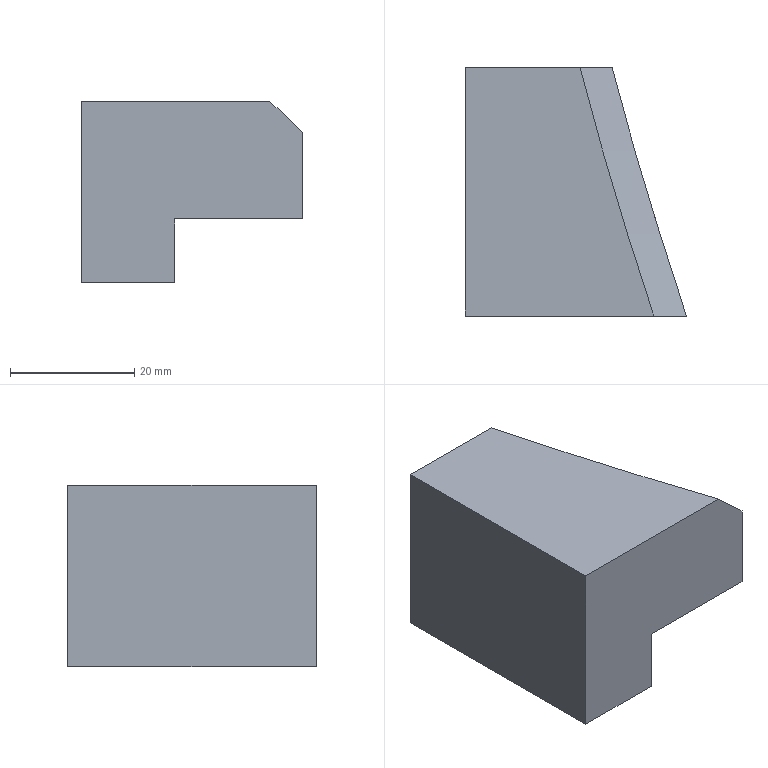Part | STEP file | Positioning_id378_x_t | 1 solid | 9 faces | box 35.628 x 40 x 29.25 mm | volume 27932 mm3 | plane 7 | spline 2
STEP:
#1=CARTESIAN_POINT('',(0.,0.,0.));
#2=DIRECTION('',(0.,0.,1.));
#3=DIRECTION('',(1.,0.,0.));
#4=AXIS2_PLACEMENT_3D('',#1,#2,#3);
#5=CARTESIAN_POINT('',(-770.37,-465.,151.245));
#6=VERTEX_POINT('',#5);
#7=CARTESIAN_POINT('',(-765.202,-465.,146.245));
#8=VERTEX_POINT('',#7);
#9=CARTESIAN_POINT('',(-770.37,-465.,151.245));
#10=CARTESIAN_POINT('',(-769.508,-465.,150.412));
#11=CARTESIAN_POINT('',(-768.647,-465.,149.578));
#12=CARTESIAN_POINT('',(-767.786,-465.,148.745));
#13=CARTESIAN_POINT('',(-766.924,-465.,147.911));
#14=CARTESIAN_POINT('',(-766.063,-465.,147.078));
#15=CARTESIAN_POINT('',(-765.202,-465.,146.245));
#16=B_SPLINE_CURVE_WITH_KNOTS('',3,(#9,#10,#11,#12,#13,#14,#15),.UNSPECIFIED.,.F.,.F.,(4,3,4),(0.,0.5,1.),.UNSPECIFIED.);
#17=CARTESIAN_POINT('',(-765.482,-463.728,146.195));
#18=CARTESIAN_POINT('',(-763.676,-470.672,146.195));
#19=CARTESIAN_POINT('',(-759.81,-484.505,146.195));
#20=CARTESIAN_POINT('',(-755.452,-498.19,146.195));
#21=CARTESIAN_POINT('',(-753.154,-504.984,146.195));
#22=CARTESIAN_POINT('',(-765.498,-463.732,146.212));
#23=CARTESIAN_POINT('',(-763.692,-470.676,146.212));
#24=CARTESIAN_POINT('',(-759.826,-484.51,146.212));
#25=CARTESIAN_POINT('',(-755.468,-498.195,146.212));
#26=CARTESIAN_POINT('',(-753.169,-504.989,146.212));
#27=CARTESIAN_POINT('',(-765.514,-463.737,146.228));
#28=CARTESIAN_POINT('',(-763.708,-470.681,146.228));
#29=CARTESIAN_POINT('',(-759.842,-484.515,146.228));
#30=CARTESIAN_POINT('',(-755.484,-498.2,146.228));
#31=CARTESIAN_POINT('',(-753.185,-504.995,146.228));
#32=CARTESIAN_POINT('',(-765.531,-463.741,146.245));
#33=CARTESIAN_POINT('',(-763.724,-470.685,146.245));
#34=CARTESIAN_POINT('',(-759.858,-484.519,146.245));
#35=CARTESIAN_POINT('',(-755.5,-498.205,146.245));
#36=CARTESIAN_POINT('',(-753.201,-505.,146.245));
#37=CARTESIAN_POINT('',(-767.144,-464.161,147.912));
#38=CARTESIAN_POINT('',(-765.332,-471.124,147.912));
#39=CARTESIAN_POINT('',(-761.455,-484.997,147.912));
#40=CARTESIAN_POINT('',(-757.085,-498.72,147.912));
#41=CARTESIAN_POINT('',(-754.78,-505.534,147.912));
#42=CARTESIAN_POINT('',(-768.757,-464.58,149.578));
#43=CARTESIAN_POINT('',(-766.94,-471.563,149.578));
#44=CARTESIAN_POINT('',(-763.052,-485.474,149.578));
#45=CARTESIAN_POINT('',(-758.67,-499.236,149.578));
#46=CARTESIAN_POINT('',(-756.358,-506.068,149.578));
#47=CARTESIAN_POINT('',(-770.37,-465.,151.245));
#48=CARTESIAN_POINT('',(-768.548,-472.002,151.245));
#49=CARTESIAN_POINT('',(-764.65,-485.951,151.245));
#50=CARTESIAN_POINT('',(-760.255,-499.751,151.245));
#51=CARTESIAN_POINT('',(-757.937,-506.602,151.245));
#52=B_SPLINE_SURFACE_WITH_KNOTS('',3,3,((#17,#18,#19,#20,#21),(#22,#23,#24,#25,#26),(#27,#28,#29,#30,#31),(#32,#33,#34,#35,#36),(#37,#38,#39,#40,#41),(#42,#43,#44,#45,#46),(#47,#48,#49,#50,#51)),.UNSPECIFIED.,.F.,.F.,.F.,(4,3,4),(4,1,4),(0.,0.009901,1.),(0.,0.5,1.),.UNSPECIFIED.);
#53=CARTESIAN_POINT('',(1.,0.));
#54=CARTESIAN_POINT('',(0.009901,0.03023));
#55=B_SPLINE_CURVE_WITH_KNOTS('',1,(#53,#54),.UNSPECIFIED.,.F.,.F.,(2,2),(0.,1.),.PIECEWISE_BEZIER_KNOTS.);
#56=(GEOMETRIC_REPRESENTATION_CONTEXT(2)PARAMETRIC_REPRESENTATION_CONTEXT()REPRESENTATION_CONTEXT('',''));
#57=DEFINITIONAL_REPRESENTATION('',(#55),#56);
#58=PCURVE('',#52,#57);
#59=CARTESIAN_POINT('',(-863.829,-465.,84.282));
#60=DIRECTION('',(0.,1.,0.));
#61=DIRECTION('',(0.,0.,-1.));
#62=AXIS2_PLACEMENT_3D('',#59,#60,#61);
#63=PLANE('',#62);
#64=CARTESIAN_POINT('',(-66.963,-93.459));
#65=CARTESIAN_POINT('',(-66.13,-94.32));
#66=CARTESIAN_POINT('',(-65.296,-95.182));
#67=CARTESIAN_POINT('',(-64.463,-96.043));
#68=CARTESIAN_POINT('',(-63.63,-96.904));
#69=CARTESIAN_POINT('',(-62.796,-97.766));
#70=CARTESIAN_POINT('',(-61.963,-98.627));
#71=B_SPLINE_CURVE_WITH_KNOTS('',3,(#64,#65,#66,#67,#68,#69,#70),.UNSPECIFIED.,.F.,.F.,(4,3,4),(0.,0.5,1.),.UNSPECIFIED.);
#72=(GEOMETRIC_REPRESENTATION_CONTEXT(2)PARAMETRIC_REPRESENTATION_CONTEXT()REPRESENTATION_CONTEXT('',''));
#73=DEFINITIONAL_REPRESENTATION('',(#71),#72);
#74=PCURVE('',#63,#73);
#75=SURFACE_CURVE('',#16,(#58,#74),.PCURVE_S1.);
#76=EDGE_CURVE('',#6,#8,#75,.T.);
#77=ORIENTED_EDGE('',*,*,#76,.F.);
#78=CARTESIAN_POINT('',(-758.477,-505.,151.245));
#79=VERTEX_POINT('',#78);
#80=CARTESIAN_POINT('',(-758.477,-505.,151.245));
#81=CARTESIAN_POINT('',(-760.597,-498.675,151.245));
#82=CARTESIAN_POINT('',(-764.802,-485.408,151.245));
#83=CARTESIAN_POINT('',(-768.548,-472.002,151.245));
#84=CARTESIAN_POINT('',(-770.37,-465.,151.245));
#85=B_SPLINE_CURVE_WITH_KNOTS('',3,(#80,#81,#82,#83,#84),.UNSPECIFIED.,.F.,.F.,(4,1,4),(0.,0.4797,1.),.UNSPECIFIED.);
#86=CARTESIAN_POINT('',(1.,0.961));
#87=CARTESIAN_POINT('',(1.,0.));
#88=B_SPLINE_CURVE_WITH_KNOTS('',1,(#86,#87),.UNSPECIFIED.,.F.,.F.,(2,2),(0.,1.),.PIECEWISE_BEZIER_KNOTS.);
#89=(GEOMETRIC_REPRESENTATION_CONTEXT(2)PARAMETRIC_REPRESENTATION_CONTEXT()REPRESENTATION_CONTEXT('',''));
#90=DEFINITIONAL_REPRESENTATION('',(#88),#89);
#91=PCURVE('',#52,#90);
#92=CARTESIAN_POINT('',(-788.829,-465.,151.245));
#93=DIRECTION('',(0.,0.,-1.));
#94=DIRECTION('',(1.,0.,0.));
#95=AXIS2_PLACEMENT_3D('',#92,#93,#94);
#96=PLANE('',#95);
#97=CARTESIAN_POINT('',(30.352,40.));
#98=CARTESIAN_POINT('',(28.232,33.675));
#99=CARTESIAN_POINT('',(24.027,20.408));
#100=CARTESIAN_POINT('',(20.281,7.002));
#101=CARTESIAN_POINT('',(18.459,-0.000000011));
#102=B_SPLINE_CURVE_WITH_KNOTS('',3,(#97,#98,#99,#100,#101),.UNSPECIFIED.,.F.,.F.,(4,1,4),(0.,0.4797,1.),.UNSPECIFIED.);
#103=(GEOMETRIC_REPRESENTATION_CONTEXT(2)PARAMETRIC_REPRESENTATION_CONTEXT()REPRESENTATION_CONTEXT('',''));
#104=DEFINITIONAL_REPRESENTATION('',(#102),#103);
#105=PCURVE('',#96,#104);
#106=SURFACE_CURVE('',#85,(#91,#105),.PCURVE_S1.);
#107=EDGE_CURVE('',#79,#6,#106,.T.);
#108=ORIENTED_EDGE('',*,*,#107,.F.);
#109=CARTESIAN_POINT('',(-753.201,-505.,146.245));
#110=VERTEX_POINT('',#109);
#111=CARTESIAN_POINT('',(-753.201,-505.,146.245));
#112=CARTESIAN_POINT('',(-754.08,-505.,147.078));
#113=CARTESIAN_POINT('',(-754.96,-505.,147.911));
#114=CARTESIAN_POINT('',(-755.839,-505.,148.745));
#115=CARTESIAN_POINT('',(-756.718,-505.,149.578));
#116=CARTESIAN_POINT('',(-757.598,-505.,150.411));
#117=CARTESIAN_POINT('',(-758.477,-505.,151.245));
#118=B_SPLINE_CURVE_WITH_KNOTS('',3,(#111,#112,#113,#114,#115,#116,#117),.UNSPECIFIED.,.F.,.F.,(4,3,4),(0.,0.5,1.),.UNSPECIFIED.);
#119=CARTESIAN_POINT('',(0.009906,1.));
#120=CARTESIAN_POINT('',(1.,0.961));
#121=B_SPLINE_CURVE_WITH_KNOTS('',1,(#119,#120),.UNSPECIFIED.,.F.,.F.,(2,2),(0.,1.),.PIECEWISE_BEZIER_KNOTS.);
#122=(GEOMETRIC_REPRESENTATION_CONTEXT(2)PARAMETRIC_REPRESENTATION_CONTEXT()REPRESENTATION_CONTEXT('',''));
#123=DEFINITIONAL_REPRESENTATION('',(#121),#122);
#124=PCURVE('',#52,#123);
#125=CARTESIAN_POINT('',(-863.829,-505.,84.282));
#126=DIRECTION('',(0.,-1.,0.));
#127=DIRECTION('',(0.,0.,1.));
#128=AXIS2_PLACEMENT_3D('',#125,#126,#127);
#129=PLANE('',#128);
#130=CARTESIAN_POINT('',(61.963,-110.628));
#131=CARTESIAN_POINT('',(62.796,-109.748));
#132=CARTESIAN_POINT('',(63.629,-108.869));
#133=CARTESIAN_POINT('',(64.463,-107.99));
#134=CARTESIAN_POINT('',(65.296,-107.11));
#135=CARTESIAN_POINT('',(66.13,-106.231));
#136=CARTESIAN_POINT('',(66.963,-105.352));
#137=B_SPLINE_CURVE_WITH_KNOTS('',3,(#130,#131,#132,#133,#134,#135,#136),.UNSPECIFIED.,.F.,.F.,(4,3,4),(0.,0.5,1.),.UNSPECIFIED.);
#138=(GEOMETRIC_REPRESENTATION_CONTEXT(2)PARAMETRIC_REPRESENTATION_CONTEXT()REPRESENTATION_CONTEXT('',''));
#139=DEFINITIONAL_REPRESENTATION('',(#137),#138);
#140=PCURVE('',#129,#139);
#141=SURFACE_CURVE('',#118,(#124,#140),.PCURVE_S1.);
#142=EDGE_CURVE('',#110,#79,#141,.T.);
#143=ORIENTED_EDGE('',*,*,#142,.F.);
#144=CARTESIAN_POINT('',(-765.202,-465.,146.245));
#145=CARTESIAN_POINT('',(-764.004,-469.56,146.245));
#146=CARTESIAN_POINT('',(-762.753,-474.107,146.245));
#147=CARTESIAN_POINT('',(-761.449,-478.638,146.245));
#148=CARTESIAN_POINT('',(-760.176,-483.061,146.245));
#149=CARTESIAN_POINT('',(-758.852,-487.47,146.245));
#150=CARTESIAN_POINT('',(-757.478,-491.863,146.245));
#151=CARTESIAN_POINT('',(-756.102,-496.258,146.245));
#152=CARTESIAN_POINT('',(-754.677,-500.638,146.245));
#153=CARTESIAN_POINT('',(-753.201,-505.,146.245));
#154=B_SPLINE_CURVE_WITH_KNOTS('',3,(#144,#145,#146,#147,#148,#149,#150,#151,#152,#153),.UNSPECIFIED.,.F.,.F.,(4,3,3,4),(0.,0.3386,0.6692,1.),.UNSPECIFIED.);
#155=CARTESIAN_POINT('',(0.009894,0.03023));
#156=CARTESIAN_POINT('',(0.009903,1.));
#157=B_SPLINE_CURVE_WITH_KNOTS('',1,(#155,#156),.UNSPECIFIED.,.F.,.F.,(2,2),(0.,1.),.PIECEWISE_BEZIER_KNOTS.);
#158=(GEOMETRIC_REPRESENTATION_CONTEXT(2)PARAMETRIC_REPRESENTATION_CONTEXT()REPRESENTATION_CONTEXT('',''));
#159=DEFINITIONAL_REPRESENTATION('',(#157),#158);
#160=PCURVE('',#52,#159);
#161=CARTESIAN_POINT('',(-753.201,-505.,146.385));
#162=CARTESIAN_POINT('',(-753.201,-505.,146.245));
#163=CARTESIAN_POINT('',(-753.201,-505.,132.282));
#164=CARTESIAN_POINT('',(-757.663,-491.811,146.385));
#165=CARTESIAN_POINT('',(-757.663,-491.811,146.245));
#166=CARTESIAN_POINT('',(-757.663,-491.811,132.282));
#167=CARTESIAN_POINT('',(-761.665,-478.472,146.385));
#168=CARTESIAN_POINT('',(-761.665,-478.472,146.245));
#169=CARTESIAN_POINT('',(-761.665,-478.472,132.282));
#170=CARTESIAN_POINT('',(-765.202,-465.,146.385));
#171=CARTESIAN_POINT('',(-765.202,-465.,146.245));
#172=CARTESIAN_POINT('',(-765.202,-465.,132.282));
#173=CARTESIAN_POINT('',(-765.237,-464.865,146.385));
#174=CARTESIAN_POINT('',(-765.237,-464.865,146.245));
#175=CARTESIAN_POINT('',(-765.237,-464.865,132.282));
#176=CARTESIAN_POINT('',(-765.272,-464.731,146.385));
#177=CARTESIAN_POINT('',(-765.272,-464.731,146.245));
#178=CARTESIAN_POINT('',(-765.272,-464.731,132.282));
#179=CARTESIAN_POINT('',(-765.308,-464.596,146.385));
#180=CARTESIAN_POINT('',(-765.308,-464.596,146.245));
#181=CARTESIAN_POINT('',(-765.308,-464.596,132.282));
#182=(BOUNDED_SURFACE()B_SPLINE_SURFACE(3,1,((#161,#162,#163),(#164,#165,#166),(#167,#168,#169),(#170,#171,#172),(#173,#174,#175),(#176,#177,#178),(#179,#180,#181)),.UNSPECIFIED.,.F.,.F.,.F.)B_SPLINE_SURFACE_WITH_KNOTS((4,3,4),(2,1,2),(0.,0.9901,1.),(0.,0.009901,1.),.UNSPECIFIED.)GEOMETRIC_REPRESENTATION_ITEM()RATIONAL_B_SPLINE_SURFACE(((0.9919,0.9919,0.9919),(0.9912,0.9912,0.9912),(0.9909,0.9909,0.9909),(0.9909,0.9909,0.9909),(0.9909,0.9909,0.9909),(0.9909,0.9909,0.9909),(0.9909,0.9909,0.9909)))REPRESENTATION_ITEM('')SURFACE());
#183=CARTESIAN_POINT('',(0.9901,0.009906));
#184=CARTESIAN_POINT('',(0.,0.009903));
#185=B_SPLINE_CURVE_WITH_KNOTS('',1,(#183,#184),.UNSPECIFIED.,.F.,.F.,(2,2),(0.,1.),.PIECEWISE_BEZIER_KNOTS.);
#186=(GEOMETRIC_REPRESENTATION_CONTEXT(2)PARAMETRIC_REPRESENTATION_CONTEXT()REPRESENTATION_CONTEXT('',''));
#187=DEFINITIONAL_REPRESENTATION('',(#185),#186);
#188=PCURVE('',#182,#187);
#189=SURFACE_CURVE('',#154,(#160,#188),.PCURVE_S1.);
#190=EDGE_CURVE('',#8,#110,#189,.T.);
#191=ORIENTED_EDGE('',*,*,#190,.F.);
#192=EDGE_LOOP('',(#77,#108,#143,#191));
#193=FACE_BOUND('',#192,.T.);
#194=ADVANCED_FACE('',(#193),#52,.T.);
#195=CARTESIAN_POINT('',(-788.829,-465.,151.245));
#196=VERTEX_POINT('',#195);
#197=CARTESIAN_POINT('',(-788.829,-505.,151.245));
#198=VERTEX_POINT('',#197);
#199=CARTESIAN_POINT('',(-788.829,-465.,151.245));
#200=DIRECTION('',(0.,-1.,0.));
#201=VECTOR('',#200,1.);
#202=LINE('',#199,#201);
#203=CARTESIAN_POINT('',(0.,0.));
#204=DIRECTION('',(0.,1.));
#205=VECTOR('',#204,1.);
#206=LINE('',#203,#205);
#207=(GEOMETRIC_REPRESENTATION_CONTEXT(2)PARAMETRIC_REPRESENTATION_CONTEXT()REPRESENTATION_CONTEXT('',''));
#208=DEFINITIONAL_REPRESENTATION('',(#206),#207);
#209=PCURVE('',#96,#208);
#210=CARTESIAN_POINT('',(-788.829,-493.037,84.282));
#211=DIRECTION('',(-1.,0.,0.));
#212=DIRECTION('',(0.,0.,-1.));
#213=AXIS2_PLACEMENT_3D('',#210,#211,#212);
#214=PLANE('',#213);
#215=CARTESIAN_POINT('',(-66.963,-28.037));
#216=DIRECTION('',(0.,1.));
#217=VECTOR('',#216,1.);
#218=LINE('',#215,#217);
#219=(GEOMETRIC_REPRESENTATION_CONTEXT(2)PARAMETRIC_REPRESENTATION_CONTEXT()REPRESENTATION_CONTEXT('',''));
#220=DEFINITIONAL_REPRESENTATION('',(#218),#219);
#221=PCURVE('',#214,#220);
#222=SURFACE_CURVE('',#202,(#209,#221),.PCURVE_S1.);
#223=EDGE_CURVE('',#196,#198,#222,.T.);
#224=ORIENTED_EDGE('',*,*,#223,.F.);
#225=CARTESIAN_POINT('',(-770.37,-465.,151.245));
#226=DIRECTION('',(-1.,0.,0.));
#227=VECTOR('',#226,1.);
#228=LINE('',#225,#227);
#229=CARTESIAN_POINT('',(18.459,0.));
#230=DIRECTION('',(-1.,0.));
#231=VECTOR('',#230,1.);
#232=LINE('',#229,#231);
#233=(GEOMETRIC_REPRESENTATION_CONTEXT(2)PARAMETRIC_REPRESENTATION_CONTEXT()REPRESENTATION_CONTEXT('',''));
#234=DEFINITIONAL_REPRESENTATION('',(#232),#233);
#235=PCURVE('',#96,#234);
#236=CARTESIAN_POINT('',(-66.963,-93.459));
#237=DIRECTION('',(0.,1.));
#238=VECTOR('',#237,1.);
#239=LINE('',#236,#238);
#240=(GEOMETRIC_REPRESENTATION_CONTEXT(2)PARAMETRIC_REPRESENTATION_CONTEXT()REPRESENTATION_CONTEXT('',''));
#241=DEFINITIONAL_REPRESENTATION('',(#239),#240);
#242=PCURVE('',#63,#241);
#243=SURFACE_CURVE('',#228,(#235,#242),.PCURVE_S1.);
#244=EDGE_CURVE('',#6,#196,#243,.T.);
#245=ORIENTED_EDGE('',*,*,#244,.F.);
#246=ORIENTED_EDGE('',*,*,#107,.F.);
#247=CARTESIAN_POINT('',(-788.829,-505.,151.245));
#248=DIRECTION('',(1.,0.,0.));
#249=VECTOR('',#248,1.);
#250=LINE('',#247,#249);
#251=CARTESIAN_POINT('',(0.,40.));
#252=DIRECTION('',(1.,0.));
#253=VECTOR('',#252,1.);
#254=LINE('',#251,#253);
#255=(GEOMETRIC_REPRESENTATION_CONTEXT(2)PARAMETRIC_REPRESENTATION_CONTEXT()REPRESENTATION_CONTEXT('',''));
#256=DEFINITIONAL_REPRESENTATION('',(#254),#255);
#257=PCURVE('',#96,#256);
#258=CARTESIAN_POINT('',(66.963,-75.));
#259=DIRECTION('',(0.,-1.));
#260=VECTOR('',#259,1.);
#261=LINE('',#258,#260);
#262=(GEOMETRIC_REPRESENTATION_CONTEXT(2)PARAMETRIC_REPRESENTATION_CONTEXT()REPRESENTATION_CONTEXT('',''));
#263=DEFINITIONAL_REPRESENTATION('',(#261),#262);
#264=PCURVE('',#129,#263);
#265=SURFACE_CURVE('',#250,(#257,#264),.PCURVE_S1.);
#266=EDGE_CURVE('',#198,#79,#265,.T.);
#267=ORIENTED_EDGE('',*,*,#266,.F.);
#268=EDGE_LOOP('',(#224,#245,#246,#267));
#269=FACE_BOUND('',#268,.F.);
#270=ADVANCED_FACE('',(#269),#96,.F.);
#271=CARTESIAN_POINT('',(-753.201,-505.,132.282));
#272=VERTEX_POINT('',#271);
#273=CARTESIAN_POINT('',(-765.202,-465.,132.282));
#274=VERTEX_POINT('',#273);
#275=CARTESIAN_POINT('',(-753.201,-505.,132.282));
#276=CARTESIAN_POINT('',(-757.663,-491.811,132.282));
#277=CARTESIAN_POINT('',(-761.665,-478.472,132.282));
#278=CARTESIAN_POINT('',(-765.202,-465.,132.282));
#279=(BOUNDED_CURVE()B_SPLINE_CURVE(3,(#275,#276,#277,#278),.UNSPECIFIED.,.F.,.F.)B_SPLINE_CURVE_WITH_KNOTS((4,4),(0.,1.),.PIECEWISE_BEZIER_KNOTS.)CURVE()GEOMETRIC_REPRESENTATION_ITEM()RATIONAL_B_SPLINE_CURVE((0.9919,0.9912,0.9909,0.9909))REPRESENTATION_ITEM(''));
#280=CARTESIAN_POINT('',(0.,1.));
#281=CARTESIAN_POINT('',(0.9901,1.));
#282=B_SPLINE_CURVE_WITH_KNOTS('',1,(#280,#281),.UNSPECIFIED.,.F.,.F.,(2,2),(0.,1.),.PIECEWISE_BEZIER_KNOTS.);
#283=(GEOMETRIC_REPRESENTATION_CONTEXT(2)PARAMETRIC_REPRESENTATION_CONTEXT()REPRESENTATION_CONTEXT('',''));
#284=DEFINITIONAL_REPRESENTATION('',(#282),#283);
#285=PCURVE('',#182,#284);
#286=CARTESIAN_POINT('',(-853.829,-493.037,132.282));
#287=DIRECTION('',(0.,0.,-1.));
#288=DIRECTION('',(1.,0.,0.));
#289=AXIS2_PLACEMENT_3D('',#286,#287,#288);
#290=PLANE('',#289);
#291=CARTESIAN_POINT('',(100.628,11.963));
#292=CARTESIAN_POINT('',(96.166,-1.226));
#293=CARTESIAN_POINT('',(92.164,-14.565));
#294=CARTESIAN_POINT('',(88.627,-28.037));
#295=(BOUNDED_CURVE()B_SPLINE_CURVE(3,(#291,#292,#293,#294),.UNSPECIFIED.,.F.,.F.)B_SPLINE_CURVE_WITH_KNOTS((4,4),(0.,1.),.PIECEWISE_BEZIER_KNOTS.)CURVE()GEOMETRIC_REPRESENTATION_ITEM()RATIONAL_B_SPLINE_CURVE((0.9919,0.9912,0.9909,0.9909))REPRESENTATION_ITEM(''));
#296=(GEOMETRIC_REPRESENTATION_CONTEXT(2)PARAMETRIC_REPRESENTATION_CONTEXT()REPRESENTATION_CONTEXT('',''));
#297=DEFINITIONAL_REPRESENTATION('',(#295),#296);
#298=PCURVE('',#290,#297);
#299=SURFACE_CURVE('',#279,(#285,#298),.PCURVE_S1.);
#300=EDGE_CURVE('',#272,#274,#299,.T.);
#301=ORIENTED_EDGE('',*,*,#300,.F.);
#302=CARTESIAN_POINT('',(-753.201,-505.,146.245));
#303=DIRECTION('',(0.,0.,-1.));
#304=VECTOR('',#303,1.);
#305=LINE('',#302,#304);
#306=CARTESIAN_POINT('',(0.,0.009901));
#307=CARTESIAN_POINT('',(0.,1.));
#308=B_SPLINE_CURVE_WITH_KNOTS('',1,(#306,#307),.UNSPECIFIED.,.F.,.F.,(2,2),(0.,13.963),.PIECEWISE_BEZIER_KNOTS.);
#309=(GEOMETRIC_REPRESENTATION_CONTEXT(2)PARAMETRIC_REPRESENTATION_CONTEXT()REPRESENTATION_CONTEXT('',''));
#310=DEFINITIONAL_REPRESENTATION('',(#308),#309);
#311=PCURVE('',#182,#310);
#312=CARTESIAN_POINT('',(61.963,-110.628));
#313=DIRECTION('',(-1.,0.));
#314=VECTOR('',#313,1.);
#315=LINE('',#312,#314);
#316=(GEOMETRIC_REPRESENTATION_CONTEXT(2)PARAMETRIC_REPRESENTATION_CONTEXT()REPRESENTATION_CONTEXT('',''));
#317=DEFINITIONAL_REPRESENTATION('',(#315),#316);
#318=PCURVE('',#129,#317);
#319=SURFACE_CURVE('',#305,(#311,#318),.PCURVE_S1.);
#320=EDGE_CURVE('',#110,#272,#319,.T.);
#321=ORIENTED_EDGE('',*,*,#320,.F.);
#322=ORIENTED_EDGE('',*,*,#190,.F.);
#323=CARTESIAN_POINT('',(-765.202,-465.,132.282));
#324=DIRECTION('',(0.,0.,1.));
#325=VECTOR('',#324,1.);
#326=LINE('',#323,#325);
#327=CARTESIAN_POINT('',(0.9901,1.));
#328=CARTESIAN_POINT('',(0.9901,0.009904));
#329=B_SPLINE_CURVE_WITH_KNOTS('',1,(#327,#328),.UNSPECIFIED.,.F.,.F.,(2,2),(0.,13.963),.PIECEWISE_BEZIER_KNOTS.);
#330=(GEOMETRIC_REPRESENTATION_CONTEXT(2)PARAMETRIC_REPRESENTATION_CONTEXT()REPRESENTATION_CONTEXT('',''));
#331=DEFINITIONAL_REPRESENTATION('',(#329),#330);
#332=PCURVE('',#182,#331);
#333=CARTESIAN_POINT('',(-48.,-98.627));
#334=DIRECTION('',(-1.,0.));
#335=VECTOR('',#334,1.);
#336=LINE('',#333,#335);
#337=(GEOMETRIC_REPRESENTATION_CONTEXT(2)PARAMETRIC_REPRESENTATION_CONTEXT()REPRESENTATION_CONTEXT('',''));
#338=DEFINITIONAL_REPRESENTATION('',(#336),#337);
#339=PCURVE('',#63,#338);
#340=SURFACE_CURVE('',#326,(#332,#339),.PCURVE_S1.);
#341=EDGE_CURVE('',#274,#8,#340,.T.);
#342=ORIENTED_EDGE('',*,*,#341,.F.);
#343=EDGE_LOOP('',(#301,#321,#322,#342));
#344=FACE_BOUND('',#343,.F.);
#345=ADVANCED_FACE('',(#344),#182,.F.);
#346=ORIENTED_EDGE('',*,*,#300,.F.);
#347=CARTESIAN_POINT('',(-773.829,-505.,132.282));
#348=VERTEX_POINT('',#347);
#349=CARTESIAN_POINT('',(-773.829,-505.,132.282));
#350=DIRECTION('',(1.,0.,0.));
#351=VECTOR('',#350,1.);
#352=LINE('',#349,#351);
#353=CARTESIAN_POINT('',(80.,11.963));
#354=DIRECTION('',(1.,0.));
#355=VECTOR('',#354,1.);
#356=LINE('',#353,#355);
#357=(GEOMETRIC_REPRESENTATION_CONTEXT(2)PARAMETRIC_REPRESENTATION_CONTEXT()REPRESENTATION_CONTEXT('',''));
#358=DEFINITIONAL_REPRESENTATION('',(#356),#357);
#359=PCURVE('',#290,#358);
#360=CARTESIAN_POINT('',(48.,-90.));
#361=DIRECTION('',(0.,-1.));
#362=VECTOR('',#361,1.);
#363=LINE('',#360,#362);
#364=(GEOMETRIC_REPRESENTATION_CONTEXT(2)PARAMETRIC_REPRESENTATION_CONTEXT()REPRESENTATION_CONTEXT('',''));
#365=DEFINITIONAL_REPRESENTATION('',(#363),#364);
#366=PCURVE('',#129,#365);
#367=SURFACE_CURVE('',#352,(#359,#366),.PCURVE_S1.);
#368=EDGE_CURVE('',#348,#272,#367,.T.);
#369=ORIENTED_EDGE('',*,*,#368,.F.);
#370=CARTESIAN_POINT('',(-773.829,-465.,132.282));
#371=VERTEX_POINT('',#370);
#372=CARTESIAN_POINT('',(-773.829,-505.,132.282));
#373=DIRECTION('',(0.,1.,0.));
#374=VECTOR('',#373,1.);
#375=LINE('',#372,#374);
#376=CARTESIAN_POINT('',(80.,11.963));
#377=DIRECTION('',(0.,-1.));
#378=VECTOR('',#377,1.);
#379=LINE('',#376,#378);
#380=(GEOMETRIC_REPRESENTATION_CONTEXT(2)PARAMETRIC_REPRESENTATION_CONTEXT()REPRESENTATION_CONTEXT('',''));
#381=DEFINITIONAL_REPRESENTATION('',(#379),#380);
#382=PCURVE('',#290,#381);
#383=CARTESIAN_POINT('',(-773.829,-463.037,135.282));
#384=DIRECTION('',(1.,0.,0.));
#385=DIRECTION('',(0.,0.,1.));
#386=AXIS2_PLACEMENT_3D('',#383,#384,#385);
#387=PLANE('',#386);
#388=CARTESIAN_POINT('',(-3.,41.963));
#389=DIRECTION('',(0.,-1.));
#390=VECTOR('',#389,1.);
#391=LINE('',#388,#390);
#392=(GEOMETRIC_REPRESENTATION_CONTEXT(2)PARAMETRIC_REPRESENTATION_CONTEXT()REPRESENTATION_CONTEXT('',''));
#393=DEFINITIONAL_REPRESENTATION('',(#391),#392);
#394=PCURVE('',#387,#393);
#395=SURFACE_CURVE('',#375,(#382,#394),.PCURVE_S1.);
#396=EDGE_CURVE('',#348,#371,#395,.T.);
#397=ORIENTED_EDGE('',*,*,#396,.T.);
#398=CARTESIAN_POINT('',(-765.202,-465.,132.282));
#399=DIRECTION('',(-1.,0.,0.));
#400=VECTOR('',#399,1.);
#401=LINE('',#398,#400);
#402=CARTESIAN_POINT('',(88.627,-28.037));
#403=DIRECTION('',(-1.,0.));
#404=VECTOR('',#403,1.);
#405=LINE('',#402,#404);
#406=(GEOMETRIC_REPRESENTATION_CONTEXT(2)PARAMETRIC_REPRESENTATION_CONTEXT()REPRESENTATION_CONTEXT('',''));
#407=DEFINITIONAL_REPRESENTATION('',(#405),#406);
#408=PCURVE('',#290,#407);
#409=CARTESIAN_POINT('',(-48.,-98.627));
#410=DIRECTION('',(0.,1.));
#411=VECTOR('',#410,1.);
#412=LINE('',#409,#411);
#413=(GEOMETRIC_REPRESENTATION_CONTEXT(2)PARAMETRIC_REPRESENTATION_CONTEXT()REPRESENTATION_CONTEXT('',''));
#414=DEFINITIONAL_REPRESENTATION('',(#412),#413);
#415=PCURVE('',#63,#414);
#416=SURFACE_CURVE('',#401,(#408,#415),.PCURVE_S1.);
#417=EDGE_CURVE('',#274,#371,#416,.T.);
#418=ORIENTED_EDGE('',*,*,#417,.F.);
#419=EDGE_LOOP('',(#346,#369,#397,#418));
#420=FACE_BOUND('',#419,.T.);
#421=ADVANCED_FACE('',(#420),#290,.T.);
#422=CARTESIAN_POINT('',(-788.829,-465.,121.995));
#423=VERTEX_POINT('',#422);
#424=CARTESIAN_POINT('',(-788.829,-465.,121.995));
#425=DIRECTION('',(0.,0.,1.));
#426=VECTOR('',#425,1.);
#427=LINE('',#424,#426);
#428=CARTESIAN_POINT('',(-37.713,-28.037));
#429=DIRECTION('',(-1.,0.));
#430=VECTOR('',#429,1.);
#431=LINE('',#428,#430);
#432=(GEOMETRIC_REPRESENTATION_CONTEXT(2)PARAMETRIC_REPRESENTATION_CONTEXT()REPRESENTATION_CONTEXT('',''));
#433=DEFINITIONAL_REPRESENTATION('',(#431),#432);
#434=PCURVE('',#214,#433);
#435=CARTESIAN_POINT('',(-37.713,-75.));
#436=DIRECTION('',(-1.,0.));
#437=VECTOR('',#436,1.);
#438=LINE('',#435,#437);
#439=(GEOMETRIC_REPRESENTATION_CONTEXT(2)PARAMETRIC_REPRESENTATION_CONTEXT()REPRESENTATION_CONTEXT('',''));
#440=DEFINITIONAL_REPRESENTATION('',(#438),#439);
#441=PCURVE('',#63,#440);
#442=SURFACE_CURVE('',#427,(#434,#441),.PCURVE_S1.);
#443=EDGE_CURVE('',#423,#196,#442,.T.);
#444=ORIENTED_EDGE('',*,*,#443,.F.);
#445=CARTESIAN_POINT('',(-788.829,-505.,121.995));
#446=VERTEX_POINT('',#445);
#447=CARTESIAN_POINT('',(-788.829,-505.,121.995));
#448=DIRECTION('',(0.,1.,0.));
#449=VECTOR('',#448,1.);
#450=LINE('',#447,#449);
#451=CARTESIAN_POINT('',(-37.713,11.963));
#452=DIRECTION('',(0.,-1.));
#453=VECTOR('',#452,1.);
#454=LINE('',#451,#453);
#455=(GEOMETRIC_REPRESENTATION_CONTEXT(2)PARAMETRIC_REPRESENTATION_CONTEXT()REPRESENTATION_CONTEXT('',''));
#456=DEFINITIONAL_REPRESENTATION('',(#454),#455);
#457=PCURVE('',#214,#456);
#458=CARTESIAN_POINT('',(-843.829,-463.037,121.995));
#459=DIRECTION('',(0.,0.,1.));
#460=DIRECTION('',(-1.,0.,0.));
#461=AXIS2_PLACEMENT_3D('',#458,#459,#460);
#462=PLANE('',#461);
#463=CARTESIAN_POINT('',(-55.,41.963));
#464=DIRECTION('',(0.,-1.));
#465=VECTOR('',#464,1.);
#466=LINE('',#463,#465);
#467=(GEOMETRIC_REPRESENTATION_CONTEXT(2)PARAMETRIC_REPRESENTATION_CONTEXT()REPRESENTATION_CONTEXT('',''));
#468=DEFINITIONAL_REPRESENTATION('',(#466),#467);
#469=PCURVE('',#462,#468);
#470=SURFACE_CURVE('',#450,(#457,#469),.PCURVE_S1.);
#471=EDGE_CURVE('',#446,#423,#470,.T.);
#472=ORIENTED_EDGE('',*,*,#471,.F.);
#473=CARTESIAN_POINT('',(-788.829,-505.,151.245));
#474=DIRECTION('',(0.,0.,-1.));
#475=VECTOR('',#474,1.);
#476=LINE('',#473,#475);
#477=CARTESIAN_POINT('',(-66.963,11.963));
#478=DIRECTION('',(1.,0.));
#479=VECTOR('',#478,1.);
#480=LINE('',#477,#479);
#481=(GEOMETRIC_REPRESENTATION_CONTEXT(2)PARAMETRIC_REPRESENTATION_CONTEXT()REPRESENTATION_CONTEXT('',''));
#482=DEFINITIONAL_REPRESENTATION('',(#480),#481);
#483=PCURVE('',#214,#482);
#484=CARTESIAN_POINT('',(66.963,-75.));
#485=DIRECTION('',(-1.,0.));
#486=VECTOR('',#485,1.);
#487=LINE('',#484,#486);
#488=(GEOMETRIC_REPRESENTATION_CONTEXT(2)PARAMETRIC_REPRESENTATION_CONTEXT()REPRESENTATION_CONTEXT('',''));
#489=DEFINITIONAL_REPRESENTATION('',(#487),#488);
#490=PCURVE('',#129,#489);
#491=SURFACE_CURVE('',#476,(#483,#490),.PCURVE_S1.);
#492=EDGE_CURVE('',#198,#446,#491,.T.);
#493=ORIENTED_EDGE('',*,*,#492,.F.);
#494=ORIENTED_EDGE('',*,*,#223,.F.);
#495=EDGE_LOOP('',(#444,#472,#493,#494));
#496=FACE_BOUND('',#495,.T.);
#497=ADVANCED_FACE('',(#496),#214,.T.);
#498=ORIENTED_EDGE('',*,*,#396,.F.);
#499=CARTESIAN_POINT('',(-773.829,-505.,121.995));
#500=VERTEX_POINT('',#499);
#501=CARTESIAN_POINT('',(-773.829,-505.,121.995));
#502=DIRECTION('',(0.,0.,1.));
#503=VECTOR('',#502,1.);
#504=LINE('',#501,#503);
#505=CARTESIAN_POINT('',(-13.287,41.963));
#506=DIRECTION('',(1.,0.));
#507=VECTOR('',#506,1.);
#508=LINE('',#505,#507);
#509=(GEOMETRIC_REPRESENTATION_CONTEXT(2)PARAMETRIC_REPRESENTATION_CONTEXT()REPRESENTATION_CONTEXT('',''));
#510=DEFINITIONAL_REPRESENTATION('',(#508),#509);
#511=PCURVE('',#387,#510);
#512=CARTESIAN_POINT('',(37.713,-90.));
#513=DIRECTION('',(1.,0.));
#514=VECTOR('',#513,1.);
#515=LINE('',#512,#514);
#516=(GEOMETRIC_REPRESENTATION_CONTEXT(2)PARAMETRIC_REPRESENTATION_CONTEXT()REPRESENTATION_CONTEXT('',''));
#517=DEFINITIONAL_REPRESENTATION('',(#515),#516);
#518=PCURVE('',#129,#517);
#519=SURFACE_CURVE('',#504,(#511,#518),.PCURVE_S1.);
#520=EDGE_CURVE('',#500,#348,#519,.T.);
#521=ORIENTED_EDGE('',*,*,#520,.F.);
#522=CARTESIAN_POINT('',(-773.829,-465.,121.995));
#523=VERTEX_POINT('',#522);
#524=CARTESIAN_POINT('',(-773.829,-465.,121.995));
#525=DIRECTION('',(0.,-1.,0.));
#526=VECTOR('',#525,1.);
#527=LINE('',#524,#526);
#528=CARTESIAN_POINT('',(-13.287,1.963));
#529=DIRECTION('',(0.,1.));
#530=VECTOR('',#529,1.);
#531=LINE('',#528,#530);
#532=(GEOMETRIC_REPRESENTATION_CONTEXT(2)PARAMETRIC_REPRESENTATION_CONTEXT()REPRESENTATION_CONTEXT('',''));
#533=DEFINITIONAL_REPRESENTATION('',(#531),#532);
#534=PCURVE('',#387,#533);
#535=CARTESIAN_POINT('',(-70.,1.963));
#536=DIRECTION('',(0.,1.));
#537=VECTOR('',#536,1.);
#538=LINE('',#535,#537);
#539=(GEOMETRIC_REPRESENTATION_CONTEXT(2)PARAMETRIC_REPRESENTATION_CONTEXT()REPRESENTATION_CONTEXT('',''));
#540=DEFINITIONAL_REPRESENTATION('',(#538),#539);
#541=PCURVE('',#462,#540);
#542=SURFACE_CURVE('',#527,(#534,#541),.PCURVE_S1.);
#543=EDGE_CURVE('',#523,#500,#542,.T.);
#544=ORIENTED_EDGE('',*,*,#543,.F.);
#545=CARTESIAN_POINT('',(-773.829,-465.,132.282));
#546=DIRECTION('',(0.,0.,-1.));
#547=VECTOR('',#546,1.);
#548=LINE('',#545,#547);
#549=CARTESIAN_POINT('',(-3.,1.963));
#550=DIRECTION('',(-1.,0.));
#551=VECTOR('',#550,1.);
#552=LINE('',#549,#551);
#553=(GEOMETRIC_REPRESENTATION_CONTEXT(2)PARAMETRIC_REPRESENTATION_CONTEXT()REPRESENTATION_CONTEXT('',''));
#554=DEFINITIONAL_REPRESENTATION('',(#552),#553);
#555=PCURVE('',#387,#554);
#556=CARTESIAN_POINT('',(-48.,-90.));
#557=DIRECTION('',(1.,0.));
#558=VECTOR('',#557,1.);
#559=LINE('',#556,#558);
#560=(GEOMETRIC_REPRESENTATION_CONTEXT(2)PARAMETRIC_REPRESENTATION_CONTEXT()REPRESENTATION_CONTEXT('',''));
#561=DEFINITIONAL_REPRESENTATION('',(#559),#560);
#562=PCURVE('',#63,#561);
#563=SURFACE_CURVE('',#548,(#555,#562),.PCURVE_S1.);
#564=EDGE_CURVE('',#371,#523,#563,.T.);
#565=ORIENTED_EDGE('',*,*,#564,.F.);
#566=EDGE_LOOP('',(#498,#521,#544,#565));
#567=FACE_BOUND('',#566,.T.);
#568=ADVANCED_FACE('',(#567),#387,.T.);
#569=ORIENTED_EDGE('',*,*,#492,.T.);
#570=CARTESIAN_POINT('',(-773.829,-505.,121.995));
#571=DIRECTION('',(-1.,0.,0.));
#572=VECTOR('',#571,1.);
#573=LINE('',#570,#572);
#574=CARTESIAN_POINT('',(37.713,-90.));
#575=DIRECTION('',(0.,1.));
#576=VECTOR('',#575,1.);
#577=LINE('',#574,#576);
#578=(GEOMETRIC_REPRESENTATION_CONTEXT(2)PARAMETRIC_REPRESENTATION_CONTEXT()REPRESENTATION_CONTEXT('',''));
#579=DEFINITIONAL_REPRESENTATION('',(#577),#578);
#580=PCURVE('',#129,#579);
#581=CARTESIAN_POINT('',(-70.,41.963));
#582=DIRECTION('',(1.,0.));
#583=VECTOR('',#582,1.);
#584=LINE('',#581,#583);
#585=(GEOMETRIC_REPRESENTATION_CONTEXT(2)PARAMETRIC_REPRESENTATION_CONTEXT()REPRESENTATION_CONTEXT('',''));
#586=DEFINITIONAL_REPRESENTATION('',(#584),#585);
#587=PCURVE('',#462,#586);
#588=SURFACE_CURVE('',#573,(#580,#587),.PCURVE_S1.);
#589=EDGE_CURVE('',#500,#446,#588,.T.);
#590=ORIENTED_EDGE('',*,*,#589,.F.);
#591=ORIENTED_EDGE('',*,*,#520,.T.);
#592=ORIENTED_EDGE('',*,*,#368,.T.);
#593=ORIENTED_EDGE('',*,*,#320,.F.);
#594=ORIENTED_EDGE('',*,*,#142,.T.);
#595=ORIENTED_EDGE('',*,*,#266,.F.);
#596=EDGE_LOOP('',(#569,#590,#591,#592,#593,#594,#595));
#597=FACE_BOUND('',#596,.T.);
#598=ADVANCED_FACE('',(#597),#129,.T.);
#599=CARTESIAN_POINT('',(-788.829,-465.,121.995));
#600=DIRECTION('',(1.,0.,0.));
#601=VECTOR('',#600,1.);
#602=LINE('',#599,#601);
#603=CARTESIAN_POINT('',(-37.713,-75.));
#604=DIRECTION('',(0.,-1.));
#605=VECTOR('',#604,1.);
#606=LINE('',#603,#605);
#607=(GEOMETRIC_REPRESENTATION_CONTEXT(2)PARAMETRIC_REPRESENTATION_CONTEXT()REPRESENTATION_CONTEXT('',''));
#608=DEFINITIONAL_REPRESENTATION('',(#606),#607);
#609=PCURVE('',#63,#608);
#610=CARTESIAN_POINT('',(-55.,1.963));
#611=DIRECTION('',(-1.,0.));
#612=VECTOR('',#611,1.);
#613=LINE('',#610,#612);
#614=(GEOMETRIC_REPRESENTATION_CONTEXT(2)PARAMETRIC_REPRESENTATION_CONTEXT()REPRESENTATION_CONTEXT('',''));
#615=DEFINITIONAL_REPRESENTATION('',(#613),#614);
#616=PCURVE('',#462,#615);
#617=SURFACE_CURVE('',#602,(#609,#616),.PCURVE_S1.);
#618=EDGE_CURVE('',#423,#523,#617,.T.);
#619=ORIENTED_EDGE('',*,*,#618,.F.);
#620=ORIENTED_EDGE('',*,*,#443,.T.);
#621=ORIENTED_EDGE('',*,*,#244,.F.);
#622=ORIENTED_EDGE('',*,*,#76,.T.);
#623=ORIENTED_EDGE('',*,*,#341,.F.);
#624=ORIENTED_EDGE('',*,*,#417,.T.);
#625=ORIENTED_EDGE('',*,*,#564,.T.);
#626=EDGE_LOOP('',(#619,#620,#621,#622,#623,#624,#625));
#627=FACE_BOUND('',#626,.T.);
#628=ADVANCED_FACE('',(#627),#63,.T.);
#629=ORIENTED_EDGE('',*,*,#589,.T.);
#630=ORIENTED_EDGE('',*,*,#471,.T.);
#631=ORIENTED_EDGE('',*,*,#618,.T.);
#632=ORIENTED_EDGE('',*,*,#543,.T.);
#633=EDGE_LOOP('',(#629,#630,#631,#632));
#634=FACE_BOUND('',#633,.T.);
#635=ADVANCED_FACE('',(#634),#462,.F.);
#636=CLOSED_SHELL('',(#194,#270,#345,#421,#497,#568,#598,#628,#635));
#637=MANIFOLD_SOLID_BREP('',#636);
#638=(LENGTH_UNIT()NAMED_UNIT(*)SI_UNIT(.MILLI.,.METRE.));
#639=UNCERTAINTY_MEASURE_WITH_UNIT(LENGTH_MEASURE(0.001),#638,'','');
#640=(NAMED_UNIT(*)PLANE_ANGLE_UNIT()SI_UNIT($,.RADIAN.));
#641=(NAMED_UNIT(*)SI_UNIT($,.STERADIAN.)SOLID_ANGLE_UNIT());
#642=(GEOMETRIC_REPRESENTATION_CONTEXT(3)GLOBAL_UNCERTAINTY_ASSIGNED_CONTEXT((#639))GLOBAL_UNIT_ASSIGNED_CONTEXT((#638,#640,#641))REPRESENTATION_CONTEXT('',''));
#643=ADVANCED_BREP_SHAPE_REPRESENTATION('',(#4,#637),#642);